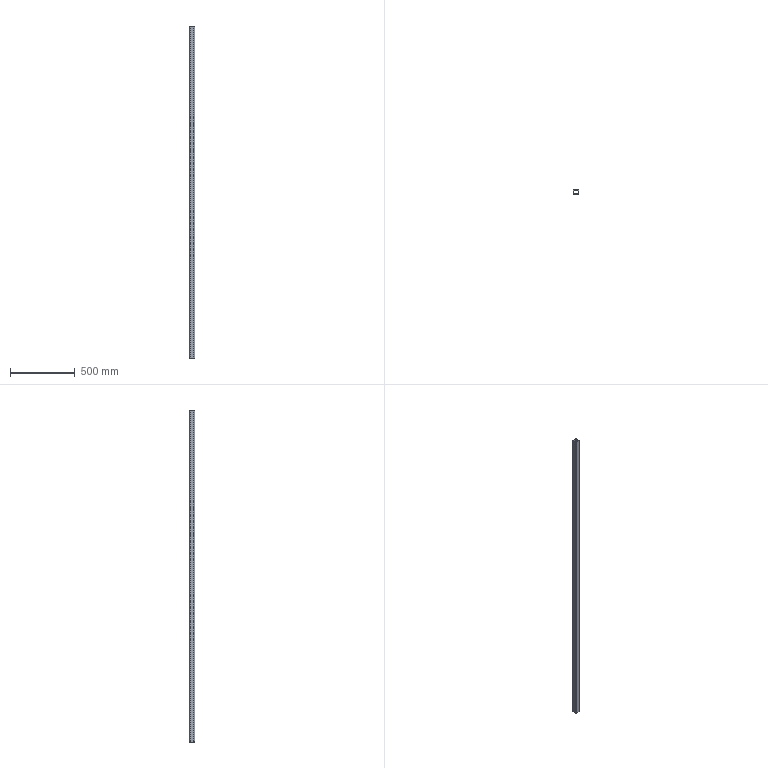Part | STEP file | body floor longitudinal beam--000.001--20240926 | 1 solid | 18 faces | box 40 x 40 x 2554 mm | volume 1074782 mm3 | plane 10 | cylinder 8 | commonest cylinder face diameters 6 x4 12 x4
STEP:
#1=CARTESIAN_POINT('',(0.,0.,0.));
#2=DIRECTION('',(0.,0.,1.));
#3=DIRECTION('',(1.,0.,0.));
#4=AXIS2_PLACEMENT_3D('',#1,#2,#3);
#5=CARTESIAN_POINT('',(-40.,149.,-50.));
#6=VERTEX_POINT('',#5);
#7=CARTESIAN_POINT('',(-40.,121.,-50.));
#8=VERTEX_POINT('',#7);
#9=CARTESIAN_POINT('',(-40.,155.,-50.));
#10=DIRECTION('',(0.,-1.,0.));
#11=VECTOR('',#10,1.);
#12=LINE('',#9,#11);
#13=CARTESIAN_POINT('',(-87.,-42.,-50.));
#14=DIRECTION('',(0.,0.,1.));
#15=DIRECTION('',(0.,-1.,0.));
#16=AXIS2_PLACEMENT_3D('',#13,#14,#15);
#17=PLANE('',#16);
#18=CARTESIAN_POINT('',(-197.,47.));
#19=DIRECTION('',(1.,0.));
#20=VECTOR('',#19,1.);
#21=LINE('',#18,#20);
#22=(GEOMETRIC_REPRESENTATION_CONTEXT(2)PARAMETRIC_REPRESENTATION_CONTEXT()REPRESENTATION_CONTEXT('',''));
#23=DEFINITIONAL_REPRESENTATION('',(#21),#22);
#24=PCURVE('',#17,#23);
#25=CARTESIAN_POINT('',(-40.,155.,2262.838));
#26=DIRECTION('',(1.,0.,0.));
#27=DIRECTION('',(0.,0.,1.));
#28=AXIS2_PLACEMENT_3D('',#25,#26,#27);
#29=PLANE('',#28);
#30=CARTESIAN_POINT('',(-2312.838,0.));
#31=DIRECTION('',(0.,1.));
#32=VECTOR('',#31,1.);
#33=LINE('',#30,#32);
#34=(GEOMETRIC_REPRESENTATION_CONTEXT(2)PARAMETRIC_REPRESENTATION_CONTEXT()REPRESENTATION_CONTEXT('',''));
#35=DEFINITIONAL_REPRESENTATION('',(#33),#34);
#36=PCURVE('',#29,#35);
#37=SURFACE_CURVE('',#12,(#24,#36),.PCURVE_S1.);
#38=EDGE_CURVE('',#6,#8,#37,.T.);
#39=ORIENTED_EDGE('',*,*,#38,.T.);
#40=CARTESIAN_POINT('',(-37.,118.,-50.));
#41=VERTEX_POINT('',#40);
#42=CARTESIAN_POINT('',(-37.,121.,-50.));
#43=DIRECTION('',(0.,0.,1.));
#44=DIRECTION('',(1.,0.,0.));
#45=AXIS2_PLACEMENT_3D('',#42,#43,#44);
#46=CIRCLE('',#45,3.);
#47=CARTESIAN_POINT('',(-163.,50.));
#48=DIRECTION('',(0.,1.));
#49=AXIS2_PLACEMENT_2D('',#47,#48);
#50=CIRCLE('',#49,3.);
#51=(GEOMETRIC_REPRESENTATION_CONTEXT(2)PARAMETRIC_REPRESENTATION_CONTEXT()REPRESENTATION_CONTEXT('',''));
#52=DEFINITIONAL_REPRESENTATION('',(#50),#51);
#53=PCURVE('',#17,#52);
#54=CARTESIAN_POINT('',(-37.,121.,2262.838));
#55=DIRECTION('',(0.,0.,1.));
#56=DIRECTION('',(-1.,0.,0.));
#57=AXIS2_PLACEMENT_3D('',#54,#55,#56);
#58=CYLINDRICAL_SURFACE('',#57,3.);
#59=CARTESIAN_POINT('',(-3.142,-2312.838));
#60=DIRECTION('',(1.,0.));
#61=VECTOR('',#60,1.);
#62=LINE('',#59,#61);
#63=(GEOMETRIC_REPRESENTATION_CONTEXT(2)PARAMETRIC_REPRESENTATION_CONTEXT()REPRESENTATION_CONTEXT('',''));
#64=DEFINITIONAL_REPRESENTATION('',(#62),#63);
#65=PCURVE('',#58,#64);
#66=SURFACE_CURVE('',#46,(#53,#65),.PCURVE_S1.);
#67=EDGE_CURVE('',#8,#41,#66,.T.);
#68=ORIENTED_EDGE('',*,*,#67,.T.);
#69=CARTESIAN_POINT('',(-9.,118.,-50.));
#70=VERTEX_POINT('',#69);
#71=CARTESIAN_POINT('',(-43.,118.,-50.));
#72=DIRECTION('',(1.,0.,0.));
#73=VECTOR('',#72,1.);
#74=LINE('',#71,#73);
#75=CARTESIAN_POINT('',(-160.,44.));
#76=DIRECTION('',(0.,1.));
#77=VECTOR('',#76,1.);
#78=LINE('',#75,#77);
#79=(GEOMETRIC_REPRESENTATION_CONTEXT(2)PARAMETRIC_REPRESENTATION_CONTEXT()REPRESENTATION_CONTEXT('',''));
#80=DEFINITIONAL_REPRESENTATION('',(#78),#79);
#81=PCURVE('',#17,#80);
#82=CARTESIAN_POINT('',(-43.,118.,2262.838));
#83=DIRECTION('',(0.,1.,0.));
#84=DIRECTION('',(0.2756,0.,-0.9613));
#85=AXIS2_PLACEMENT_3D('',#82,#83,#84);
#86=PLANE('',#85);
#87=CARTESIAN_POINT('',(2223.243,637.505));
#88=DIRECTION('',(0.2756,-0.9613));
#89=VECTOR('',#88,1.);
#90=LINE('',#87,#89);
#91=(GEOMETRIC_REPRESENTATION_CONTEXT(2)PARAMETRIC_REPRESENTATION_CONTEXT()REPRESENTATION_CONTEXT('',''));
#92=DEFINITIONAL_REPRESENTATION('',(#90),#91);
#93=PCURVE('',#86,#92);
#94=SURFACE_CURVE('',#74,(#81,#93),.PCURVE_S1.);
#95=EDGE_CURVE('',#41,#70,#94,.T.);
#96=ORIENTED_EDGE('',*,*,#95,.T.);
#97=CARTESIAN_POINT('',(-6.,121.,-50.));
#98=VERTEX_POINT('',#97);
#99=CARTESIAN_POINT('',(-9.,121.,-50.));
#100=DIRECTION('',(0.,0.,1.));
#101=DIRECTION('',(1.,0.,0.));
#102=AXIS2_PLACEMENT_3D('',#99,#100,#101);
#103=CIRCLE('',#102,3.);
#104=CARTESIAN_POINT('',(-163.,78.));
#105=DIRECTION('',(0.,1.));
#106=AXIS2_PLACEMENT_2D('',#104,#105);
#107=CIRCLE('',#106,3.);
#108=(GEOMETRIC_REPRESENTATION_CONTEXT(2)PARAMETRIC_REPRESENTATION_CONTEXT()REPRESENTATION_CONTEXT('',''));
#109=DEFINITIONAL_REPRESENTATION('',(#107),#108);
#110=PCURVE('',#17,#109);
#111=CARTESIAN_POINT('',(-9.,121.,2262.838));
#112=DIRECTION('',(0.,0.,1.));
#113=DIRECTION('',(-1.,0.,0.));
#114=AXIS2_PLACEMENT_3D('',#111,#112,#113);
#115=CYLINDRICAL_SURFACE('',#114,3.);
#116=CARTESIAN_POINT('',(-3.142,-2312.838));
#117=DIRECTION('',(1.,0.));
#118=VECTOR('',#117,1.);
#119=LINE('',#116,#118);
#120=(GEOMETRIC_REPRESENTATION_CONTEXT(2)PARAMETRIC_REPRESENTATION_CONTEXT()REPRESENTATION_CONTEXT('',''));
#121=DEFINITIONAL_REPRESENTATION('',(#119),#120);
#122=PCURVE('',#115,#121);
#123=SURFACE_CURVE('',#103,(#110,#122),.PCURVE_S1.);
#124=EDGE_CURVE('',#70,#98,#123,.T.);
#125=ORIENTED_EDGE('',*,*,#124,.T.);
#126=CARTESIAN_POINT('',(-6.,149.,-50.));
#127=VERTEX_POINT('',#126);
#128=CARTESIAN_POINT('',(-6.,115.,-50.));
#129=DIRECTION('',(0.,1.,0.));
#130=VECTOR('',#129,1.);
#131=LINE('',#128,#130);
#132=CARTESIAN_POINT('',(-157.,81.));
#133=DIRECTION('',(-1.,0.));
#134=VECTOR('',#133,1.);
#135=LINE('',#132,#134);
#136=(GEOMETRIC_REPRESENTATION_CONTEXT(2)PARAMETRIC_REPRESENTATION_CONTEXT()REPRESENTATION_CONTEXT('',''));
#137=DEFINITIONAL_REPRESENTATION('',(#135),#136);
#138=PCURVE('',#17,#137);
#139=CARTESIAN_POINT('',(-6.,115.,2262.838));
#140=DIRECTION('',(-1.,0.,0.));
#141=DIRECTION('',(0.,0.,-1.));
#142=AXIS2_PLACEMENT_3D('',#139,#140,#141);
#143=PLANE('',#142);
#144=CARTESIAN_POINT('',(2312.838,0.));
#145=DIRECTION('',(0.,-1.));
#146=VECTOR('',#145,1.);
#147=LINE('',#144,#146);
#148=(GEOMETRIC_REPRESENTATION_CONTEXT(2)PARAMETRIC_REPRESENTATION_CONTEXT()REPRESENTATION_CONTEXT('',''));
#149=DEFINITIONAL_REPRESENTATION('',(#147),#148);
#150=PCURVE('',#143,#149);
#151=SURFACE_CURVE('',#131,(#138,#150),.PCURVE_S1.);
#152=EDGE_CURVE('',#98,#127,#151,.T.);
#153=ORIENTED_EDGE('',*,*,#152,.T.);
#154=CARTESIAN_POINT('',(-9.,152.,-50.));
#155=VERTEX_POINT('',#154);
#156=CARTESIAN_POINT('',(-9.,149.,-50.));
#157=DIRECTION('',(0.,0.,1.));
#158=DIRECTION('',(1.,0.,0.));
#159=AXIS2_PLACEMENT_3D('',#156,#157,#158);
#160=CIRCLE('',#159,3.);
#161=CARTESIAN_POINT('',(-191.,78.));
#162=DIRECTION('',(0.,1.));
#163=AXIS2_PLACEMENT_2D('',#161,#162);
#164=CIRCLE('',#163,3.);
#165=(GEOMETRIC_REPRESENTATION_CONTEXT(2)PARAMETRIC_REPRESENTATION_CONTEXT()REPRESENTATION_CONTEXT('',''));
#166=DEFINITIONAL_REPRESENTATION('',(#164),#165);
#167=PCURVE('',#17,#166);
#168=CARTESIAN_POINT('',(-9.,149.,2262.838));
#169=DIRECTION('',(0.,0.,1.));
#170=DIRECTION('',(-1.,0.,0.));
#171=AXIS2_PLACEMENT_3D('',#168,#169,#170);
#172=CYLINDRICAL_SURFACE('',#171,3.);
#173=CARTESIAN_POINT('',(3.142,-2312.838));
#174=DIRECTION('',(1.,0.));
#175=VECTOR('',#174,1.);
#176=LINE('',#173,#175);
#177=(GEOMETRIC_REPRESENTATION_CONTEXT(2)PARAMETRIC_REPRESENTATION_CONTEXT()REPRESENTATION_CONTEXT('',''));
#178=DEFINITIONAL_REPRESENTATION('',(#176),#177);
#179=PCURVE('',#172,#178);
#180=SURFACE_CURVE('',#160,(#167,#179),.PCURVE_S1.);
#181=EDGE_CURVE('',#127,#155,#180,.T.);
#182=ORIENTED_EDGE('',*,*,#181,.T.);
#183=CARTESIAN_POINT('',(-37.,152.,-50.));
#184=VERTEX_POINT('',#183);
#185=CARTESIAN_POINT('',(-3.,152.,-50.));
#186=DIRECTION('',(-1.,0.,0.));
#187=VECTOR('',#186,1.);
#188=LINE('',#185,#187);
#189=CARTESIAN_POINT('',(-194.,84.));
#190=DIRECTION('',(0.,-1.));
#191=VECTOR('',#190,1.);
#192=LINE('',#189,#191);
#193=(GEOMETRIC_REPRESENTATION_CONTEXT(2)PARAMETRIC_REPRESENTATION_CONTEXT()REPRESENTATION_CONTEXT('',''));
#194=DEFINITIONAL_REPRESENTATION('',(#192),#193);
#195=PCURVE('',#17,#194);
#196=CARTESIAN_POINT('',(-3.,152.,2262.838));
#197=DIRECTION('',(0.,-1.,0.));
#198=DIRECTION('',(-0.2756,0.,0.9613));
#199=AXIS2_PLACEMENT_3D('',#196,#197,#198);
#200=PLANE('',#199);
#201=CARTESIAN_POINT('',(-2223.243,637.505));
#202=DIRECTION('',(0.2756,0.9613));
#203=VECTOR('',#202,1.);
#204=LINE('',#201,#203);
#205=(GEOMETRIC_REPRESENTATION_CONTEXT(2)PARAMETRIC_REPRESENTATION_CONTEXT()REPRESENTATION_CONTEXT('',''));
#206=DEFINITIONAL_REPRESENTATION('',(#204),#205);
#207=PCURVE('',#200,#206);
#208=SURFACE_CURVE('',#188,(#195,#207),.PCURVE_S1.);
#209=EDGE_CURVE('',#155,#184,#208,.T.);
#210=ORIENTED_EDGE('',*,*,#209,.T.);
#211=CARTESIAN_POINT('',(-37.,149.,-50.));
#212=DIRECTION('',(0.,0.,1.));
#213=DIRECTION('',(1.,0.,0.));
#214=AXIS2_PLACEMENT_3D('',#211,#212,#213);
#215=CIRCLE('',#214,3.);
#216=CARTESIAN_POINT('',(-191.,50.));
#217=DIRECTION('',(0.,1.));
#218=AXIS2_PLACEMENT_2D('',#216,#217);
#219=CIRCLE('',#218,3.);
#220=(GEOMETRIC_REPRESENTATION_CONTEXT(2)PARAMETRIC_REPRESENTATION_CONTEXT()REPRESENTATION_CONTEXT('',''));
#221=DEFINITIONAL_REPRESENTATION('',(#219),#220);
#222=PCURVE('',#17,#221);
#223=CARTESIAN_POINT('',(-37.,149.,2262.838));
#224=DIRECTION('',(0.,0.,1.));
#225=DIRECTION('',(-1.,0.,0.));
#226=AXIS2_PLACEMENT_3D('',#223,#224,#225);
#227=CYLINDRICAL_SURFACE('',#226,3.);
#228=CARTESIAN_POINT('',(3.142,-2312.838));
#229=DIRECTION('',(1.,0.));
#230=VECTOR('',#229,1.);
#231=LINE('',#228,#230);
#232=(GEOMETRIC_REPRESENTATION_CONTEXT(2)PARAMETRIC_REPRESENTATION_CONTEXT()REPRESENTATION_CONTEXT('',''));
#233=DEFINITIONAL_REPRESENTATION('',(#231),#232);
#234=PCURVE('',#227,#233);
#235=SURFACE_CURVE('',#215,(#222,#234),.PCURVE_S1.);
#236=EDGE_CURVE('',#184,#6,#235,.T.);
#237=ORIENTED_EDGE('',*,*,#236,.T.);
#238=EDGE_LOOP('',(#39,#68,#96,#125,#153,#182,#210,#237));
#239=FACE_BOUND('',#238,.T.);
#240=CARTESIAN_POINT('',(-3.,121.,-50.));
#241=VERTEX_POINT('',#240);
#242=CARTESIAN_POINT('',(-3.,149.,-50.));
#243=VERTEX_POINT('',#242);
#244=CARTESIAN_POINT('',(-3.,115.,-50.));
#245=DIRECTION('',(0.,1.,0.));
#246=VECTOR('',#245,1.);
#247=LINE('',#244,#246);
#248=CARTESIAN_POINT('',(-157.,84.));
#249=DIRECTION('',(-1.,0.));
#250=VECTOR('',#249,1.);
#251=LINE('',#248,#250);
#252=(GEOMETRIC_REPRESENTATION_CONTEXT(2)PARAMETRIC_REPRESENTATION_CONTEXT()REPRESENTATION_CONTEXT('',''));
#253=DEFINITIONAL_REPRESENTATION('',(#251),#252);
#254=PCURVE('',#17,#253);
#255=CARTESIAN_POINT('',(-3.,115.,2262.838));
#256=DIRECTION('',(-1.,0.,0.));
#257=DIRECTION('',(0.,0.,-1.));
#258=AXIS2_PLACEMENT_3D('',#255,#256,#257);
#259=PLANE('',#258);
#260=CARTESIAN_POINT('',(2312.838,0.));
#261=DIRECTION('',(0.,-1.));
#262=VECTOR('',#261,1.);
#263=LINE('',#260,#262);
#264=(GEOMETRIC_REPRESENTATION_CONTEXT(2)PARAMETRIC_REPRESENTATION_CONTEXT()REPRESENTATION_CONTEXT('',''));
#265=DEFINITIONAL_REPRESENTATION('',(#263),#264);
#266=PCURVE('',#259,#265);
#267=SURFACE_CURVE('',#247,(#254,#266),.PCURVE_S1.);
#268=EDGE_CURVE('',#241,#243,#267,.T.);
#269=ORIENTED_EDGE('',*,*,#268,.F.);
#270=CARTESIAN_POINT('',(-9.,115.,-50.));
#271=VERTEX_POINT('',#270);
#272=CARTESIAN_POINT('',(-9.,121.,-50.));
#273=DIRECTION('',(0.,0.,-1.));
#274=DIRECTION('',(1.,0.,0.));
#275=AXIS2_PLACEMENT_3D('',#272,#273,#274);
#276=CIRCLE('',#275,6.);
#277=CARTESIAN_POINT('',(-163.,84.));
#278=CARTESIAN_POINT('',(-152.608,84.));
#279=CARTESIAN_POINT('',(-157.804,75.));
#280=CARTESIAN_POINT('',(-163.,66.));
#281=CARTESIAN_POINT('',(-168.196,75.));
#282=CARTESIAN_POINT('',(-173.392,84.));
#283=CARTESIAN_POINT('',(-163.,84.));
#284=(BOUNDED_CURVE()B_SPLINE_CURVE(2,(#277,#278,#279,#280,#281,#282,#283),.UNSPECIFIED.,.T.,.F.)B_SPLINE_CURVE_WITH_KNOTS((1,2,2,2,2,1),(-2.094,0.,2.094,4.189,6.283,8.378),.UNSPECIFIED.)CURVE()GEOMETRIC_REPRESENTATION_ITEM()RATIONAL_B_SPLINE_CURVE((1.,0.5,1.,0.5,1.,0.5,1.))REPRESENTATION_ITEM(''));
#285=(GEOMETRIC_REPRESENTATION_CONTEXT(2)PARAMETRIC_REPRESENTATION_CONTEXT()REPRESENTATION_CONTEXT('',''));
#286=DEFINITIONAL_REPRESENTATION('',(#284),#285);
#287=PCURVE('',#17,#286);
#288=CARTESIAN_POINT('',(-9.,121.,2262.838));
#289=DIRECTION('',(0.,0.,1.));
#290=DIRECTION('',(-1.,0.,0.));
#291=AXIS2_PLACEMENT_3D('',#288,#289,#290);
#292=CYLINDRICAL_SURFACE('',#291,6.);
#293=CARTESIAN_POINT('',(3.142,-2312.838));
#294=DIRECTION('',(-1.,0.));
#295=VECTOR('',#294,1.);
#296=LINE('',#293,#295);
#297=(GEOMETRIC_REPRESENTATION_CONTEXT(2)PARAMETRIC_REPRESENTATION_CONTEXT()REPRESENTATION_CONTEXT('',''));
#298=DEFINITIONAL_REPRESENTATION('',(#296),#297);
#299=PCURVE('',#292,#298);
#300=SURFACE_CURVE('',#276,(#287,#299),.PCURVE_S1.);
#301=EDGE_CURVE('',#241,#271,#300,.T.);
#302=ORIENTED_EDGE('',*,*,#301,.T.);
#303=CARTESIAN_POINT('',(-37.,115.,-50.));
#304=VERTEX_POINT('',#303);
#305=CARTESIAN_POINT('',(-43.,115.,-50.));
#306=DIRECTION('',(1.,0.,0.));
#307=VECTOR('',#306,1.);
#308=LINE('',#305,#307);
#309=CARTESIAN_POINT('',(-157.,44.));
#310=DIRECTION('',(0.,1.));
#311=VECTOR('',#310,1.);
#312=LINE('',#309,#311);
#313=(GEOMETRIC_REPRESENTATION_CONTEXT(2)PARAMETRIC_REPRESENTATION_CONTEXT()REPRESENTATION_CONTEXT('',''));
#314=DEFINITIONAL_REPRESENTATION('',(#312),#313);
#315=PCURVE('',#17,#314);
#316=CARTESIAN_POINT('',(-43.,115.,2262.838));
#317=DIRECTION('',(0.,1.,0.));
#318=DIRECTION('',(0.2756,0.,-0.9613));
#319=AXIS2_PLACEMENT_3D('',#316,#317,#318);
#320=PLANE('',#319);
#321=CARTESIAN_POINT('',(2223.243,637.505));
#322=DIRECTION('',(0.2756,-0.9613));
#323=VECTOR('',#322,1.);
#324=LINE('',#321,#323);
#325=(GEOMETRIC_REPRESENTATION_CONTEXT(2)PARAMETRIC_REPRESENTATION_CONTEXT()REPRESENTATION_CONTEXT('',''));
#326=DEFINITIONAL_REPRESENTATION('',(#324),#325);
#327=PCURVE('',#320,#326);
#328=SURFACE_CURVE('',#308,(#315,#327),.PCURVE_S1.);
#329=EDGE_CURVE('',#304,#271,#328,.T.);
#330=ORIENTED_EDGE('',*,*,#329,.F.);
#331=CARTESIAN_POINT('',(-43.,121.,-50.));
#332=VERTEX_POINT('',#331);
#333=CARTESIAN_POINT('',(-37.,121.,-50.));
#334=DIRECTION('',(0.,0.,-1.));
#335=DIRECTION('',(1.,0.,0.));
#336=AXIS2_PLACEMENT_3D('',#333,#334,#335);
#337=CIRCLE('',#336,6.);
#338=CARTESIAN_POINT('',(-163.,56.));
#339=CARTESIAN_POINT('',(-152.608,56.));
#340=CARTESIAN_POINT('',(-157.804,47.));
#341=CARTESIAN_POINT('',(-163.,38.));
#342=CARTESIAN_POINT('',(-168.196,47.));
#343=CARTESIAN_POINT('',(-173.392,56.));
#344=CARTESIAN_POINT('',(-163.,56.));
#345=(BOUNDED_CURVE()B_SPLINE_CURVE(2,(#338,#339,#340,#341,#342,#343,#344),.UNSPECIFIED.,.T.,.F.)B_SPLINE_CURVE_WITH_KNOTS((1,2,2,2,2,1),(-2.094,0.,2.094,4.189,6.283,8.378),.UNSPECIFIED.)CURVE()GEOMETRIC_REPRESENTATION_ITEM()RATIONAL_B_SPLINE_CURVE((1.,0.5,1.,0.5,1.,0.5,1.))REPRESENTATION_ITEM(''));
#346=(GEOMETRIC_REPRESENTATION_CONTEXT(2)PARAMETRIC_REPRESENTATION_CONTEXT()REPRESENTATION_CONTEXT('',''));
#347=DEFINITIONAL_REPRESENTATION('',(#345),#346);
#348=PCURVE('',#17,#347);
#349=CARTESIAN_POINT('',(-37.,121.,2262.838));
#350=DIRECTION('',(0.,0.,1.));
#351=DIRECTION('',(-1.,0.,0.));
#352=AXIS2_PLACEMENT_3D('',#349,#350,#351);
#353=CYLINDRICAL_SURFACE('',#352,6.);
#354=CARTESIAN_POINT('',(3.142,-2312.838));
#355=DIRECTION('',(-1.,0.));
#356=VECTOR('',#355,1.);
#357=LINE('',#354,#356);
#358=(GEOMETRIC_REPRESENTATION_CONTEXT(2)PARAMETRIC_REPRESENTATION_CONTEXT()REPRESENTATION_CONTEXT('',''));
#359=DEFINITIONAL_REPRESENTATION('',(#357),#358);
#360=PCURVE('',#353,#359);
#361=SURFACE_CURVE('',#337,(#348,#360),.PCURVE_S1.);
#362=EDGE_CURVE('',#304,#332,#361,.T.);
#363=ORIENTED_EDGE('',*,*,#362,.T.);
#364=CARTESIAN_POINT('',(-43.,149.,-50.));
#365=VERTEX_POINT('',#364);
#366=CARTESIAN_POINT('',(-43.,155.,-50.));
#367=DIRECTION('',(0.,-1.,0.));
#368=VECTOR('',#367,1.);
#369=LINE('',#366,#368);
#370=CARTESIAN_POINT('',(-197.,44.));
#371=DIRECTION('',(1.,0.));
#372=VECTOR('',#371,1.);
#373=LINE('',#370,#372);
#374=(GEOMETRIC_REPRESENTATION_CONTEXT(2)PARAMETRIC_REPRESENTATION_CONTEXT()REPRESENTATION_CONTEXT('',''));
#375=DEFINITIONAL_REPRESENTATION('',(#373),#374);
#376=PCURVE('',#17,#375);
#377=CARTESIAN_POINT('',(-43.,155.,2262.838));
#378=DIRECTION('',(1.,0.,0.));
#379=DIRECTION('',(0.,0.,1.));
#380=AXIS2_PLACEMENT_3D('',#377,#378,#379);
#381=PLANE('',#380);
#382=CARTESIAN_POINT('',(-2312.838,0.));
#383=DIRECTION('',(0.,1.));
#384=VECTOR('',#383,1.);
#385=LINE('',#382,#384);
#386=(GEOMETRIC_REPRESENTATION_CONTEXT(2)PARAMETRIC_REPRESENTATION_CONTEXT()REPRESENTATION_CONTEXT('',''));
#387=DEFINITIONAL_REPRESENTATION('',(#385),#386);
#388=PCURVE('',#381,#387);
#389=SURFACE_CURVE('',#369,(#376,#388),.PCURVE_S1.);
#390=EDGE_CURVE('',#365,#332,#389,.T.);
#391=ORIENTED_EDGE('',*,*,#390,.F.);
#392=CARTESIAN_POINT('',(-37.,155.,-50.));
#393=VERTEX_POINT('',#392);
#394=CARTESIAN_POINT('',(-37.,149.,-50.));
#395=DIRECTION('',(0.,0.,-1.));
#396=DIRECTION('',(1.,0.,0.));
#397=AXIS2_PLACEMENT_3D('',#394,#395,#396);
#398=CIRCLE('',#397,6.);
#399=CARTESIAN_POINT('',(-191.,56.));
#400=CARTESIAN_POINT('',(-180.608,56.));
#401=CARTESIAN_POINT('',(-185.804,47.));
#402=CARTESIAN_POINT('',(-191.,38.));
#403=CARTESIAN_POINT('',(-196.196,47.));
#404=CARTESIAN_POINT('',(-201.392,56.));
#405=CARTESIAN_POINT('',(-191.,56.));
#406=(BOUNDED_CURVE()B_SPLINE_CURVE(2,(#399,#400,#401,#402,#403,#404,#405),.UNSPECIFIED.,.T.,.F.)B_SPLINE_CURVE_WITH_KNOTS((1,2,2,2,2,1),(-2.094,0.,2.094,4.189,6.283,8.378),.UNSPECIFIED.)CURVE()GEOMETRIC_REPRESENTATION_ITEM()RATIONAL_B_SPLINE_CURVE((1.,0.5,1.,0.5,1.,0.5,1.))REPRESENTATION_ITEM(''));
#407=(GEOMETRIC_REPRESENTATION_CONTEXT(2)PARAMETRIC_REPRESENTATION_CONTEXT()REPRESENTATION_CONTEXT('',''));
#408=DEFINITIONAL_REPRESENTATION('',(#406),#407);
#409=PCURVE('',#17,#408);
#410=CARTESIAN_POINT('',(-37.,149.,2262.838));
#411=DIRECTION('',(0.,0.,1.));
#412=DIRECTION('',(-1.,0.,0.));
#413=AXIS2_PLACEMENT_3D('',#410,#411,#412);
#414=CYLINDRICAL_SURFACE('',#413,6.);
#415=CARTESIAN_POINT('',(9.425,-2312.838));
#416=DIRECTION('',(-1.,0.));
#417=VECTOR('',#416,1.);
#418=LINE('',#415,#417);
#419=(GEOMETRIC_REPRESENTATION_CONTEXT(2)PARAMETRIC_REPRESENTATION_CONTEXT()REPRESENTATION_CONTEXT('',''));
#420=DEFINITIONAL_REPRESENTATION('',(#418),#419);
#421=PCURVE('',#414,#420);
#422=SURFACE_CURVE('',#398,(#409,#421),.PCURVE_S1.);
#423=EDGE_CURVE('',#365,#393,#422,.T.);
#424=ORIENTED_EDGE('',*,*,#423,.T.);
#425=CARTESIAN_POINT('',(-9.,155.,-50.));
#426=VERTEX_POINT('',#425);
#427=CARTESIAN_POINT('',(-3.,155.,-50.));
#428=DIRECTION('',(-1.,0.,0.));
#429=VECTOR('',#428,1.);
#430=LINE('',#427,#429);
#431=CARTESIAN_POINT('',(-197.,84.));
#432=DIRECTION('',(0.,-1.));
#433=VECTOR('',#432,1.);
#434=LINE('',#431,#433);
#435=(GEOMETRIC_REPRESENTATION_CONTEXT(2)PARAMETRIC_REPRESENTATION_CONTEXT()REPRESENTATION_CONTEXT('',''));
#436=DEFINITIONAL_REPRESENTATION('',(#434),#435);
#437=PCURVE('',#17,#436);
#438=CARTESIAN_POINT('',(-3.,155.,2262.838));
#439=DIRECTION('',(0.,-1.,0.));
#440=DIRECTION('',(-0.2756,0.,0.9613));
#441=AXIS2_PLACEMENT_3D('',#438,#439,#440);
#442=PLANE('',#441);
#443=CARTESIAN_POINT('',(-2223.243,637.505));
#444=DIRECTION('',(0.2756,0.9613));
#445=VECTOR('',#444,1.);
#446=LINE('',#443,#445);
#447=(GEOMETRIC_REPRESENTATION_CONTEXT(2)PARAMETRIC_REPRESENTATION_CONTEXT()REPRESENTATION_CONTEXT('',''));
#448=DEFINITIONAL_REPRESENTATION('',(#446),#447);
#449=PCURVE('',#442,#448);
#450=SURFACE_CURVE('',#430,(#437,#449),.PCURVE_S1.);
#451=EDGE_CURVE('',#426,#393,#450,.T.);
#452=ORIENTED_EDGE('',*,*,#451,.F.);
#453=CARTESIAN_POINT('',(-9.,149.,-50.));
#454=DIRECTION('',(0.,0.,-1.));
#455=DIRECTION('',(1.,0.,0.));
#456=AXIS2_PLACEMENT_3D('',#453,#454,#455);
#457=CIRCLE('',#456,6.);
#458=CARTESIAN_POINT('',(-191.,84.));
#459=CARTESIAN_POINT('',(-180.608,84.));
#460=CARTESIAN_POINT('',(-185.804,75.));
#461=CARTESIAN_POINT('',(-191.,66.));
#462=CARTESIAN_POINT('',(-196.196,75.));
#463=CARTESIAN_POINT('',(-201.392,84.));
#464=CARTESIAN_POINT('',(-191.,84.));
#465=(BOUNDED_CURVE()B_SPLINE_CURVE(2,(#458,#459,#460,#461,#462,#463,#464),.UNSPECIFIED.,.T.,.F.)B_SPLINE_CURVE_WITH_KNOTS((1,2,2,2,2,1),(-2.094,0.,2.094,4.189,6.283,8.378),.UNSPECIFIED.)CURVE()GEOMETRIC_REPRESENTATION_ITEM()RATIONAL_B_SPLINE_CURVE((1.,0.5,1.,0.5,1.,0.5,1.))REPRESENTATION_ITEM(''));
#466=(GEOMETRIC_REPRESENTATION_CONTEXT(2)PARAMETRIC_REPRESENTATION_CONTEXT()REPRESENTATION_CONTEXT('',''));
#467=DEFINITIONAL_REPRESENTATION('',(#465),#466);
#468=PCURVE('',#17,#467);
#469=CARTESIAN_POINT('',(-9.,149.,2262.838));
#470=DIRECTION('',(0.,0.,1.));
#471=DIRECTION('',(-1.,0.,0.));
#472=AXIS2_PLACEMENT_3D('',#469,#470,#471);
#473=CYLINDRICAL_SURFACE('',#472,6.);
#474=CARTESIAN_POINT('',(9.425,-2312.838));
#475=DIRECTION('',(-1.,0.));
#476=VECTOR('',#475,1.);
#477=LINE('',#474,#476);
#478=(GEOMETRIC_REPRESENTATION_CONTEXT(2)PARAMETRIC_REPRESENTATION_CONTEXT()REPRESENTATION_CONTEXT('',''));
#479=DEFINITIONAL_REPRESENTATION('',(#477),#478);
#480=PCURVE('',#473,#479);
#481=SURFACE_CURVE('',#457,(#468,#480),.PCURVE_S1.);
#482=EDGE_CURVE('',#426,#243,#481,.T.);
#483=ORIENTED_EDGE('',*,*,#482,.T.);
#484=EDGE_LOOP('',(#269,#302,#330,#363,#391,#424,#452,#483));
#485=FACE_BOUND('',#484,.T.);
#486=ADVANCED_FACE('',(#239,#485),#17,.F.);
#487=CARTESIAN_POINT('',(-37.,118.,2504.));
#488=VERTEX_POINT('',#487);
#489=CARTESIAN_POINT('',(-9.,118.,2504.));
#490=VERTEX_POINT('',#489);
#491=CARTESIAN_POINT('',(-43.,118.,2504.));
#492=DIRECTION('',(1.,0.,0.));
#493=VECTOR('',#492,1.);
#494=LINE('',#491,#493);
#495=CARTESIAN_POINT('',(-112.,92.,2504.));
#496=DIRECTION('',(0.,0.,1.));
#497=DIRECTION('',(0.,1.,0.));
#498=AXIS2_PLACEMENT_3D('',#495,#496,#497);
#499=PLANE('',#498);
#500=CARTESIAN_POINT('',(26.,-69.));
#501=DIRECTION('',(0.,-1.));
#502=VECTOR('',#501,1.);
#503=LINE('',#500,#502);
#504=(GEOMETRIC_REPRESENTATION_CONTEXT(2)PARAMETRIC_REPRESENTATION_CONTEXT()REPRESENTATION_CONTEXT('',''));
#505=DEFINITIONAL_REPRESENTATION('',(#503),#504);
#506=PCURVE('',#499,#505);
#507=CARTESIAN_POINT('',(-231.819,-66.473));
#508=DIRECTION('',(0.2756,-0.9613));
#509=VECTOR('',#508,1.);
#510=LINE('',#507,#509);
#511=(GEOMETRIC_REPRESENTATION_CONTEXT(2)PARAMETRIC_REPRESENTATION_CONTEXT()REPRESENTATION_CONTEXT('',''));
#512=DEFINITIONAL_REPRESENTATION('',(#510),#511);
#513=PCURVE('',#86,#512);
#514=SURFACE_CURVE('',#494,(#506,#513),.PCURVE_S1.);
#515=EDGE_CURVE('',#488,#490,#514,.T.);
#516=ORIENTED_EDGE('',*,*,#515,.F.);
#517=CARTESIAN_POINT('',(-40.,121.,2504.));
#518=VERTEX_POINT('',#517);
#519=CARTESIAN_POINT('',(-37.,121.,2504.));
#520=DIRECTION('',(0.,0.,-1.));
#521=DIRECTION('',(1.,0.,0.));
#522=AXIS2_PLACEMENT_3D('',#519,#520,#521);
#523=CIRCLE('',#522,3.);
#524=CARTESIAN_POINT('',(29.,-78.));
#525=CARTESIAN_POINT('',(23.804,-78.));
#526=CARTESIAN_POINT('',(26.402,-73.5));
#527=CARTESIAN_POINT('',(29.,-69.));
#528=CARTESIAN_POINT('',(31.598,-73.5));
#529=CARTESIAN_POINT('',(34.196,-78.));
#530=CARTESIAN_POINT('',(29.,-78.));
#531=(BOUNDED_CURVE()B_SPLINE_CURVE(2,(#524,#525,#526,#527,#528,#529,#530),.UNSPECIFIED.,.T.,.F.)B_SPLINE_CURVE_WITH_KNOTS((1,2,2,2,2,1),(-2.094,0.,2.094,4.189,6.283,8.378),.UNSPECIFIED.)CURVE()GEOMETRIC_REPRESENTATION_ITEM()RATIONAL_B_SPLINE_CURVE((1.,0.5,1.,0.5,1.,0.5,1.))REPRESENTATION_ITEM(''));
#532=(GEOMETRIC_REPRESENTATION_CONTEXT(2)PARAMETRIC_REPRESENTATION_CONTEXT()REPRESENTATION_CONTEXT('',''));
#533=DEFINITIONAL_REPRESENTATION('',(#531),#532);
#534=PCURVE('',#499,#533);
#535=CARTESIAN_POINT('',(3.142,241.162));
#536=DIRECTION('',(-1.,0.));
#537=VECTOR('',#536,1.);
#538=LINE('',#535,#537);
#539=(GEOMETRIC_REPRESENTATION_CONTEXT(2)PARAMETRIC_REPRESENTATION_CONTEXT()REPRESENTATION_CONTEXT('',''));
#540=DEFINITIONAL_REPRESENTATION('',(#538),#539);
#541=PCURVE('',#58,#540);
#542=SURFACE_CURVE('',#523,(#534,#541),.PCURVE_S1.);
#543=EDGE_CURVE('',#488,#518,#542,.T.);
#544=ORIENTED_EDGE('',*,*,#543,.T.);
#545=CARTESIAN_POINT('',(-40.,149.,2504.));
#546=VERTEX_POINT('',#545);
#547=CARTESIAN_POINT('',(-40.,155.,2504.));
#548=DIRECTION('',(0.,-1.,0.));
#549=VECTOR('',#548,1.);
#550=LINE('',#547,#549);
#551=CARTESIAN_POINT('',(63.,-72.));
#552=DIRECTION('',(-1.,0.));
#553=VECTOR('',#552,1.);
#554=LINE('',#551,#553);
#555=(GEOMETRIC_REPRESENTATION_CONTEXT(2)PARAMETRIC_REPRESENTATION_CONTEXT()REPRESENTATION_CONTEXT('',''));
#556=DEFINITIONAL_REPRESENTATION('',(#554),#555);
#557=PCURVE('',#499,#556);
#558=CARTESIAN_POINT('',(241.162,0.));
#559=DIRECTION('',(0.,1.));
#560=VECTOR('',#559,1.);
#561=LINE('',#558,#560);
#562=(GEOMETRIC_REPRESENTATION_CONTEXT(2)PARAMETRIC_REPRESENTATION_CONTEXT()REPRESENTATION_CONTEXT('',''));
#563=DEFINITIONAL_REPRESENTATION('',(#561),#562);
#564=PCURVE('',#29,#563);
#565=SURFACE_CURVE('',#550,(#557,#564),.PCURVE_S1.);
#566=EDGE_CURVE('',#546,#518,#565,.T.);
#567=ORIENTED_EDGE('',*,*,#566,.F.);
#568=CARTESIAN_POINT('',(-37.,152.,2504.));
#569=VERTEX_POINT('',#568);
#570=CARTESIAN_POINT('',(-37.,149.,2504.));
#571=DIRECTION('',(0.,0.,-1.));
#572=DIRECTION('',(1.,0.,0.));
#573=AXIS2_PLACEMENT_3D('',#570,#571,#572);
#574=CIRCLE('',#573,3.);
#575=CARTESIAN_POINT('',(57.,-78.));
#576=CARTESIAN_POINT('',(51.804,-78.));
#577=CARTESIAN_POINT('',(54.402,-73.5));
#578=CARTESIAN_POINT('',(57.,-69.));
#579=CARTESIAN_POINT('',(59.598,-73.5));
#580=CARTESIAN_POINT('',(62.196,-78.));
#581=CARTESIAN_POINT('',(57.,-78.));
#582=(BOUNDED_CURVE()B_SPLINE_CURVE(2,(#575,#576,#577,#578,#579,#580,#581),.UNSPECIFIED.,.T.,.F.)B_SPLINE_CURVE_WITH_KNOTS((1,2,2,2,2,1),(-2.094,0.,2.094,4.189,6.283,8.378),.UNSPECIFIED.)CURVE()GEOMETRIC_REPRESENTATION_ITEM()RATIONAL_B_SPLINE_CURVE((1.,0.5,1.,0.5,1.,0.5,1.))REPRESENTATION_ITEM(''));
#583=(GEOMETRIC_REPRESENTATION_CONTEXT(2)PARAMETRIC_REPRESENTATION_CONTEXT()REPRESENTATION_CONTEXT('',''));
#584=DEFINITIONAL_REPRESENTATION('',(#582),#583);
#585=PCURVE('',#499,#584);
#586=CARTESIAN_POINT('',(9.425,241.162));
#587=DIRECTION('',(-1.,0.));
#588=VECTOR('',#587,1.);
#589=LINE('',#586,#588);
#590=(GEOMETRIC_REPRESENTATION_CONTEXT(2)PARAMETRIC_REPRESENTATION_CONTEXT()REPRESENTATION_CONTEXT('',''));
#591=DEFINITIONAL_REPRESENTATION('',(#589),#590);
#592=PCURVE('',#227,#591);
#593=SURFACE_CURVE('',#574,(#585,#592),.PCURVE_S1.);
#594=EDGE_CURVE('',#546,#569,#593,.T.);
#595=ORIENTED_EDGE('',*,*,#594,.T.);
#596=CARTESIAN_POINT('',(-9.,152.,2504.));
#597=VERTEX_POINT('',#596);
#598=CARTESIAN_POINT('',(-3.,152.,2504.));
#599=DIRECTION('',(-1.,0.,0.));
#600=VECTOR('',#599,1.);
#601=LINE('',#598,#600);
#602=CARTESIAN_POINT('',(60.,-109.));
#603=DIRECTION('',(0.,1.));
#604=VECTOR('',#603,1.);
#605=LINE('',#602,#604);
#606=(GEOMETRIC_REPRESENTATION_CONTEXT(2)PARAMETRIC_REPRESENTATION_CONTEXT()REPRESENTATION_CONTEXT('',''));
#607=DEFINITIONAL_REPRESENTATION('',(#605),#606);
#608=PCURVE('',#499,#607);
#609=CARTESIAN_POINT('',(231.819,-66.473));
#610=DIRECTION('',(0.2756,0.9613));
#611=VECTOR('',#610,1.);
#612=LINE('',#609,#611);
#613=(GEOMETRIC_REPRESENTATION_CONTEXT(2)PARAMETRIC_REPRESENTATION_CONTEXT()REPRESENTATION_CONTEXT('',''));
#614=DEFINITIONAL_REPRESENTATION('',(#612),#613);
#615=PCURVE('',#200,#614);
#616=SURFACE_CURVE('',#601,(#608,#615),.PCURVE_S1.);
#617=EDGE_CURVE('',#597,#569,#616,.T.);
#618=ORIENTED_EDGE('',*,*,#617,.F.);
#619=CARTESIAN_POINT('',(-6.,149.,2504.));
#620=VERTEX_POINT('',#619);
#621=CARTESIAN_POINT('',(-9.,149.,2504.));
#622=DIRECTION('',(0.,0.,-1.));
#623=DIRECTION('',(1.,0.,0.));
#624=AXIS2_PLACEMENT_3D('',#621,#622,#623);
#625=CIRCLE('',#624,3.);
#626=CARTESIAN_POINT('',(57.,-106.));
#627=CARTESIAN_POINT('',(51.804,-106.));
#628=CARTESIAN_POINT('',(54.402,-101.5));
#629=CARTESIAN_POINT('',(57.,-97.));
#630=CARTESIAN_POINT('',(59.598,-101.5));
#631=CARTESIAN_POINT('',(62.196,-106.));
#632=CARTESIAN_POINT('',(57.,-106.));
#633=(BOUNDED_CURVE()B_SPLINE_CURVE(2,(#626,#627,#628,#629,#630,#631,#632),.UNSPECIFIED.,.T.,.F.)B_SPLINE_CURVE_WITH_KNOTS((1,2,2,2,2,1),(-2.094,0.,2.094,4.189,6.283,8.378),.UNSPECIFIED.)CURVE()GEOMETRIC_REPRESENTATION_ITEM()RATIONAL_B_SPLINE_CURVE((1.,0.5,1.,0.5,1.,0.5,1.))REPRESENTATION_ITEM(''));
#634=(GEOMETRIC_REPRESENTATION_CONTEXT(2)PARAMETRIC_REPRESENTATION_CONTEXT()REPRESENTATION_CONTEXT('',''));
#635=DEFINITIONAL_REPRESENTATION('',(#633),#634);
#636=PCURVE('',#499,#635);
#637=CARTESIAN_POINT('',(9.425,241.162));
#638=DIRECTION('',(-1.,0.));
#639=VECTOR('',#638,1.);
#640=LINE('',#637,#639);
#641=(GEOMETRIC_REPRESENTATION_CONTEXT(2)PARAMETRIC_REPRESENTATION_CONTEXT()REPRESENTATION_CONTEXT('',''));
#642=DEFINITIONAL_REPRESENTATION('',(#640),#641);
#643=PCURVE('',#172,#642);
#644=SURFACE_CURVE('',#625,(#636,#643),.PCURVE_S1.);
#645=EDGE_CURVE('',#597,#620,#644,.T.);
#646=ORIENTED_EDGE('',*,*,#645,.T.);
#647=CARTESIAN_POINT('',(-6.,121.,2504.));
#648=VERTEX_POINT('',#647);
#649=CARTESIAN_POINT('',(-6.,115.,2504.));
#650=DIRECTION('',(0.,1.,0.));
#651=VECTOR('',#650,1.);
#652=LINE('',#649,#651);
#653=CARTESIAN_POINT('',(23.,-106.));
#654=DIRECTION('',(1.,0.));
#655=VECTOR('',#654,1.);
#656=LINE('',#653,#655);
#657=(GEOMETRIC_REPRESENTATION_CONTEXT(2)PARAMETRIC_REPRESENTATION_CONTEXT()REPRESENTATION_CONTEXT('',''));
#658=DEFINITIONAL_REPRESENTATION('',(#656),#657);
#659=PCURVE('',#499,#658);
#660=CARTESIAN_POINT('',(-241.162,0.));
#661=DIRECTION('',(0.,-1.));
#662=VECTOR('',#661,1.);
#663=LINE('',#660,#662);
#664=(GEOMETRIC_REPRESENTATION_CONTEXT(2)PARAMETRIC_REPRESENTATION_CONTEXT()REPRESENTATION_CONTEXT('',''));
#665=DEFINITIONAL_REPRESENTATION('',(#663),#664);
#666=PCURVE('',#143,#665);
#667=SURFACE_CURVE('',#652,(#659,#666),.PCURVE_S1.);
#668=EDGE_CURVE('',#648,#620,#667,.T.);
#669=ORIENTED_EDGE('',*,*,#668,.F.);
#670=CARTESIAN_POINT('',(-9.,121.,2504.));
#671=DIRECTION('',(0.,0.,-1.));
#672=DIRECTION('',(1.,0.,0.));
#673=AXIS2_PLACEMENT_3D('',#670,#671,#672);
#674=CIRCLE('',#673,3.);
#675=CARTESIAN_POINT('',(29.,-106.));
#676=CARTESIAN_POINT('',(23.804,-106.));
#677=CARTESIAN_POINT('',(26.402,-101.5));
#678=CARTESIAN_POINT('',(29.,-97.));
#679=CARTESIAN_POINT('',(31.598,-101.5));
#680=CARTESIAN_POINT('',(34.196,-106.));
#681=CARTESIAN_POINT('',(29.,-106.));
#682=(BOUNDED_CURVE()B_SPLINE_CURVE(2,(#675,#676,#677,#678,#679,#680,#681),.UNSPECIFIED.,.T.,.F.)B_SPLINE_CURVE_WITH_KNOTS((1,2,2,2,2,1),(-2.094,0.,2.094,4.189,6.283,8.378),.UNSPECIFIED.)CURVE()GEOMETRIC_REPRESENTATION_ITEM()RATIONAL_B_SPLINE_CURVE((1.,0.5,1.,0.5,1.,0.5,1.))REPRESENTATION_ITEM(''));
#683=(GEOMETRIC_REPRESENTATION_CONTEXT(2)PARAMETRIC_REPRESENTATION_CONTEXT()REPRESENTATION_CONTEXT('',''));
#684=DEFINITIONAL_REPRESENTATION('',(#682),#683);
#685=PCURVE('',#499,#684);
#686=CARTESIAN_POINT('',(3.142,241.162));
#687=DIRECTION('',(-1.,0.));
#688=VECTOR('',#687,1.);
#689=LINE('',#686,#688);
#690=(GEOMETRIC_REPRESENTATION_CONTEXT(2)PARAMETRIC_REPRESENTATION_CONTEXT()REPRESENTATION_CONTEXT('',''));
#691=DEFINITIONAL_REPRESENTATION('',(#689),#690);
#692=PCURVE('',#115,#691);
#693=SURFACE_CURVE('',#674,(#685,#692),.PCURVE_S1.);
#694=EDGE_CURVE('',#648,#490,#693,.T.);
#695=ORIENTED_EDGE('',*,*,#694,.T.);
#696=EDGE_LOOP('',(#516,#544,#567,#595,#618,#646,#669,#695));
#697=FACE_BOUND('',#696,.T.);
#698=CARTESIAN_POINT('',(-37.,115.,2504.));
#699=VERTEX_POINT('',#698);
#700=CARTESIAN_POINT('',(-9.,115.,2504.));
#701=VERTEX_POINT('',#700);
#702=CARTESIAN_POINT('',(-43.,115.,2504.));
#703=DIRECTION('',(1.,0.,0.));
#704=VECTOR('',#703,1.);
#705=LINE('',#702,#704);
#706=CARTESIAN_POINT('',(23.,-69.));
#707=DIRECTION('',(0.,-1.));
#708=VECTOR('',#707,1.);
#709=LINE('',#706,#708);
#710=(GEOMETRIC_REPRESENTATION_CONTEXT(2)PARAMETRIC_REPRESENTATION_CONTEXT()REPRESENTATION_CONTEXT('',''));
#711=DEFINITIONAL_REPRESENTATION('',(#709),#710);
#712=PCURVE('',#499,#711);
#713=CARTESIAN_POINT('',(-231.819,-66.473));
#714=DIRECTION('',(0.2756,-0.9613));
#715=VECTOR('',#714,1.);
#716=LINE('',#713,#715);
#717=(GEOMETRIC_REPRESENTATION_CONTEXT(2)PARAMETRIC_REPRESENTATION_CONTEXT()REPRESENTATION_CONTEXT('',''));
#718=DEFINITIONAL_REPRESENTATION('',(#716),#717);
#719=PCURVE('',#320,#718);
#720=SURFACE_CURVE('',#705,(#712,#719),.PCURVE_S1.);
#721=EDGE_CURVE('',#699,#701,#720,.T.);
#722=ORIENTED_EDGE('',*,*,#721,.T.);
#723=CARTESIAN_POINT('',(-3.,121.,2504.));
#724=VERTEX_POINT('',#723);
#725=CARTESIAN_POINT('',(-9.,121.,2504.));
#726=DIRECTION('',(0.,0.,1.));
#727=DIRECTION('',(1.,0.,0.));
#728=AXIS2_PLACEMENT_3D('',#725,#726,#727);
#729=CIRCLE('',#728,6.);
#730=CARTESIAN_POINT('',(29.,-103.));
#731=DIRECTION('',(0.,-1.));
#732=AXIS2_PLACEMENT_2D('',#730,#731);
#733=CIRCLE('',#732,6.);
#734=(GEOMETRIC_REPRESENTATION_CONTEXT(2)PARAMETRIC_REPRESENTATION_CONTEXT()REPRESENTATION_CONTEXT('',''));
#735=DEFINITIONAL_REPRESENTATION('',(#733),#734);
#736=PCURVE('',#499,#735);
#737=CARTESIAN_POINT('',(-3.142,241.162));
#738=DIRECTION('',(1.,0.));
#739=VECTOR('',#738,1.);
#740=LINE('',#737,#739);
#741=(GEOMETRIC_REPRESENTATION_CONTEXT(2)PARAMETRIC_REPRESENTATION_CONTEXT()REPRESENTATION_CONTEXT('',''));
#742=DEFINITIONAL_REPRESENTATION('',(#740),#741);
#743=PCURVE('',#292,#742);
#744=SURFACE_CURVE('',#729,(#736,#743),.PCURVE_S1.);
#745=EDGE_CURVE('',#701,#724,#744,.T.);
#746=ORIENTED_EDGE('',*,*,#745,.T.);
#747=CARTESIAN_POINT('',(-3.,149.,2504.));
#748=VERTEX_POINT('',#747);
#749=CARTESIAN_POINT('',(-3.,115.,2504.));
#750=DIRECTION('',(0.,1.,0.));
#751=VECTOR('',#750,1.);
#752=LINE('',#749,#751);
#753=CARTESIAN_POINT('',(23.,-109.));
#754=DIRECTION('',(1.,0.));
#755=VECTOR('',#754,1.);
#756=LINE('',#753,#755);
#757=(GEOMETRIC_REPRESENTATION_CONTEXT(2)PARAMETRIC_REPRESENTATION_CONTEXT()REPRESENTATION_CONTEXT('',''));
#758=DEFINITIONAL_REPRESENTATION('',(#756),#757);
#759=PCURVE('',#499,#758);
#760=CARTESIAN_POINT('',(-241.162,0.));
#761=DIRECTION('',(0.,-1.));
#762=VECTOR('',#761,1.);
#763=LINE('',#760,#762);
#764=(GEOMETRIC_REPRESENTATION_CONTEXT(2)PARAMETRIC_REPRESENTATION_CONTEXT()REPRESENTATION_CONTEXT('',''));
#765=DEFINITIONAL_REPRESENTATION('',(#763),#764);
#766=PCURVE('',#259,#765);
#767=SURFACE_CURVE('',#752,(#759,#766),.PCURVE_S1.);
#768=EDGE_CURVE('',#724,#748,#767,.T.);
#769=ORIENTED_EDGE('',*,*,#768,.T.);
#770=CARTESIAN_POINT('',(-9.,155.,2504.));
#771=VERTEX_POINT('',#770);
#772=CARTESIAN_POINT('',(-9.,149.,2504.));
#773=DIRECTION('',(0.,0.,1.));
#774=DIRECTION('',(1.,0.,0.));
#775=AXIS2_PLACEMENT_3D('',#772,#773,#774);
#776=CIRCLE('',#775,6.);
#777=CARTESIAN_POINT('',(57.,-103.));
#778=DIRECTION('',(0.,-1.));
#779=AXIS2_PLACEMENT_2D('',#777,#778);
#780=CIRCLE('',#779,6.);
#781=(GEOMETRIC_REPRESENTATION_CONTEXT(2)PARAMETRIC_REPRESENTATION_CONTEXT()REPRESENTATION_CONTEXT('',''));
#782=DEFINITIONAL_REPRESENTATION('',(#780),#781);
#783=PCURVE('',#499,#782);
#784=CARTESIAN_POINT('',(3.142,241.162));
#785=DIRECTION('',(1.,0.));
#786=VECTOR('',#785,1.);
#787=LINE('',#784,#786);
#788=(GEOMETRIC_REPRESENTATION_CONTEXT(2)PARAMETRIC_REPRESENTATION_CONTEXT()REPRESENTATION_CONTEXT('',''));
#789=DEFINITIONAL_REPRESENTATION('',(#787),#788);
#790=PCURVE('',#473,#789);
#791=SURFACE_CURVE('',#776,(#783,#790),.PCURVE_S1.);
#792=EDGE_CURVE('',#748,#771,#791,.T.);
#793=ORIENTED_EDGE('',*,*,#792,.T.);
#794=CARTESIAN_POINT('',(-37.,155.,2504.));
#795=VERTEX_POINT('',#794);
#796=CARTESIAN_POINT('',(-3.,155.,2504.));
#797=DIRECTION('',(-1.,0.,0.));
#798=VECTOR('',#797,1.);
#799=LINE('',#796,#798);
#800=CARTESIAN_POINT('',(63.,-109.));
#801=DIRECTION('',(0.,1.));
#802=VECTOR('',#801,1.);
#803=LINE('',#800,#802);
#804=(GEOMETRIC_REPRESENTATION_CONTEXT(2)PARAMETRIC_REPRESENTATION_CONTEXT()REPRESENTATION_CONTEXT('',''));
#805=DEFINITIONAL_REPRESENTATION('',(#803),#804);
#806=PCURVE('',#499,#805);
#807=CARTESIAN_POINT('',(231.819,-66.473));
#808=DIRECTION('',(0.2756,0.9613));
#809=VECTOR('',#808,1.);
#810=LINE('',#807,#809);
#811=(GEOMETRIC_REPRESENTATION_CONTEXT(2)PARAMETRIC_REPRESENTATION_CONTEXT()REPRESENTATION_CONTEXT('',''));
#812=DEFINITIONAL_REPRESENTATION('',(#810),#811);
#813=PCURVE('',#442,#812);
#814=SURFACE_CURVE('',#799,(#806,#813),.PCURVE_S1.);
#815=EDGE_CURVE('',#771,#795,#814,.T.);
#816=ORIENTED_EDGE('',*,*,#815,.T.);
#817=CARTESIAN_POINT('',(-43.,149.,2504.));
#818=VERTEX_POINT('',#817);
#819=CARTESIAN_POINT('',(-37.,149.,2504.));
#820=DIRECTION('',(0.,0.,1.));
#821=DIRECTION('',(1.,0.,0.));
#822=AXIS2_PLACEMENT_3D('',#819,#820,#821);
#823=CIRCLE('',#822,6.);
#824=CARTESIAN_POINT('',(57.,-75.));
#825=DIRECTION('',(0.,-1.));
#826=AXIS2_PLACEMENT_2D('',#824,#825);
#827=CIRCLE('',#826,6.);
#828=(GEOMETRIC_REPRESENTATION_CONTEXT(2)PARAMETRIC_REPRESENTATION_CONTEXT()REPRESENTATION_CONTEXT('',''));
#829=DEFINITIONAL_REPRESENTATION('',(#827),#828);
#830=PCURVE('',#499,#829);
#831=CARTESIAN_POINT('',(3.142,241.162));
#832=DIRECTION('',(1.,0.));
#833=VECTOR('',#832,1.);
#834=LINE('',#831,#833);
#835=(GEOMETRIC_REPRESENTATION_CONTEXT(2)PARAMETRIC_REPRESENTATION_CONTEXT()REPRESENTATION_CONTEXT('',''));
#836=DEFINITIONAL_REPRESENTATION('',(#834),#835);
#837=PCURVE('',#414,#836);
#838=SURFACE_CURVE('',#823,(#830,#837),.PCURVE_S1.);
#839=EDGE_CURVE('',#795,#818,#838,.T.);
#840=ORIENTED_EDGE('',*,*,#839,.T.);
#841=CARTESIAN_POINT('',(-43.,121.,2504.));
#842=VERTEX_POINT('',#841);
#843=CARTESIAN_POINT('',(-43.,155.,2504.));
#844=DIRECTION('',(0.,-1.,0.));
#845=VECTOR('',#844,1.);
#846=LINE('',#843,#845);
#847=CARTESIAN_POINT('',(63.,-69.));
#848=DIRECTION('',(-1.,0.));
#849=VECTOR('',#848,1.);
#850=LINE('',#847,#849);
#851=(GEOMETRIC_REPRESENTATION_CONTEXT(2)PARAMETRIC_REPRESENTATION_CONTEXT()REPRESENTATION_CONTEXT('',''));
#852=DEFINITIONAL_REPRESENTATION('',(#850),#851);
#853=PCURVE('',#499,#852);
#854=CARTESIAN_POINT('',(241.162,0.));
#855=DIRECTION('',(0.,1.));
#856=VECTOR('',#855,1.);
#857=LINE('',#854,#856);
#858=(GEOMETRIC_REPRESENTATION_CONTEXT(2)PARAMETRIC_REPRESENTATION_CONTEXT()REPRESENTATION_CONTEXT('',''));
#859=DEFINITIONAL_REPRESENTATION('',(#857),#858);
#860=PCURVE('',#381,#859);
#861=SURFACE_CURVE('',#846,(#853,#860),.PCURVE_S1.);
#862=EDGE_CURVE('',#818,#842,#861,.T.);
#863=ORIENTED_EDGE('',*,*,#862,.T.);
#864=CARTESIAN_POINT('',(-37.,121.,2504.));
#865=DIRECTION('',(0.,0.,1.));
#866=DIRECTION('',(1.,0.,0.));
#867=AXIS2_PLACEMENT_3D('',#864,#865,#866);
#868=CIRCLE('',#867,6.);
#869=CARTESIAN_POINT('',(29.,-75.));
#870=DIRECTION('',(0.,-1.));
#871=AXIS2_PLACEMENT_2D('',#869,#870);
#872=CIRCLE('',#871,6.);
#873=(GEOMETRIC_REPRESENTATION_CONTEXT(2)PARAMETRIC_REPRESENTATION_CONTEXT()REPRESENTATION_CONTEXT('',''));
#874=DEFINITIONAL_REPRESENTATION('',(#872),#873);
#875=PCURVE('',#499,#874);
#876=CARTESIAN_POINT('',(-3.142,241.162));
#877=DIRECTION('',(1.,0.));
#878=VECTOR('',#877,1.);
#879=LINE('',#876,#878);
#880=(GEOMETRIC_REPRESENTATION_CONTEXT(2)PARAMETRIC_REPRESENTATION_CONTEXT()REPRESENTATION_CONTEXT('',''));
#881=DEFINITIONAL_REPRESENTATION('',(#879),#880);
#882=PCURVE('',#353,#881);
#883=SURFACE_CURVE('',#868,(#875,#882),.PCURVE_S1.);
#884=EDGE_CURVE('',#842,#699,#883,.T.);
#885=ORIENTED_EDGE('',*,*,#884,.T.);
#886=EDGE_LOOP('',(#722,#746,#769,#793,#816,#840,#863,#885));
#887=FACE_BOUND('',#886,.T.);
#888=ADVANCED_FACE('',(#697,#887),#499,.T.);
#889=ORIENTED_EDGE('',*,*,#95,.F.);
#890=CARTESIAN_POINT('',(-37.,118.,2504.));
#891=DIRECTION('',(0.,0.,1.));
#892=VECTOR('',#891,1.);
#893=LINE('',#890,#892);
#894=CARTESIAN_POINT('',(-230.166,-72.241));
#895=DIRECTION('',(-0.9613,-0.2756));
#896=VECTOR('',#895,1.);
#897=LINE('',#894,#896);
#898=(GEOMETRIC_REPRESENTATION_CONTEXT(2)PARAMETRIC_REPRESENTATION_CONTEXT()REPRESENTATION_CONTEXT('',''));
#899=DEFINITIONAL_REPRESENTATION('',(#897),#898);
#900=PCURVE('',#86,#899);
#901=CARTESIAN_POINT('',(1.571,241.162));
#902=DIRECTION('',(0.,1.));
#903=VECTOR('',#902,1.);
#904=LINE('',#901,#903);
#905=(GEOMETRIC_REPRESENTATION_CONTEXT(2)PARAMETRIC_REPRESENTATION_CONTEXT()REPRESENTATION_CONTEXT('',''));
#906=DEFINITIONAL_REPRESENTATION('',(#904),#905);
#907=PCURVE('',#58,#906);
#908=SURFACE_CURVE('',#893,(#900,#907),.PCURVE_S1.);
#909=EDGE_CURVE('',#41,#488,#908,.T.);
#910=ORIENTED_EDGE('',*,*,#909,.T.);
#911=ORIENTED_EDGE('',*,*,#515,.T.);
#912=CARTESIAN_POINT('',(-9.,118.,0.));
#913=DIRECTION('',(0.,0.,-1.));
#914=VECTOR('',#913,1.);
#915=LINE('',#912,#914);
#916=CARTESIAN_POINT('',(2184.552,591.04));
#917=DIRECTION('',(0.9613,0.2756));
#918=VECTOR('',#917,1.);
#919=LINE('',#916,#918);
#920=(GEOMETRIC_REPRESENTATION_CONTEXT(2)PARAMETRIC_REPRESENTATION_CONTEXT()REPRESENTATION_CONTEXT('',''));
#921=DEFINITIONAL_REPRESENTATION('',(#919),#920);
#922=PCURVE('',#86,#921);
#923=CARTESIAN_POINT('',(1.571,-2262.838));
#924=DIRECTION('',(0.,-1.));
#925=VECTOR('',#924,1.);
#926=LINE('',#923,#925);
#927=(GEOMETRIC_REPRESENTATION_CONTEXT(2)PARAMETRIC_REPRESENTATION_CONTEXT()REPRESENTATION_CONTEXT('',''));
#928=DEFINITIONAL_REPRESENTATION('',(#926),#927);
#929=PCURVE('',#115,#928);
#930=SURFACE_CURVE('',#915,(#922,#929),.PCURVE_S1.);
#931=EDGE_CURVE('',#490,#70,#930,.T.);
#932=ORIENTED_EDGE('',*,*,#931,.T.);
#933=EDGE_LOOP('',(#889,#910,#911,#932));
#934=FACE_BOUND('',#933,.T.);
#935=ADVANCED_FACE('',(#934),#86,.T.);
#936=ORIENTED_EDGE('',*,*,#152,.F.);
#937=CARTESIAN_POINT('',(-6.,121.,2504.));
#938=DIRECTION('',(0.,0.,1.));
#939=VECTOR('',#938,1.);
#940=LINE('',#937,#939);
#941=CARTESIAN_POINT('',(-241.162,-6.));
#942=DIRECTION('',(-1.,0.));
#943=VECTOR('',#942,1.);
#944=LINE('',#941,#943);
#945=(GEOMETRIC_REPRESENTATION_CONTEXT(2)PARAMETRIC_REPRESENTATION_CONTEXT()REPRESENTATION_CONTEXT('',''));
#946=DEFINITIONAL_REPRESENTATION('',(#944),#945);
#947=PCURVE('',#143,#946);
#948=CARTESIAN_POINT('',(3.142,241.162));
#949=DIRECTION('',(0.,1.));
#950=VECTOR('',#949,1.);
#951=LINE('',#948,#950);
#952=(GEOMETRIC_REPRESENTATION_CONTEXT(2)PARAMETRIC_REPRESENTATION_CONTEXT()REPRESENTATION_CONTEXT('',''));
#953=DEFINITIONAL_REPRESENTATION('',(#951),#952);
#954=PCURVE('',#115,#953);
#955=SURFACE_CURVE('',#940,(#947,#954),.PCURVE_S1.);
#956=EDGE_CURVE('',#98,#648,#955,.T.);
#957=ORIENTED_EDGE('',*,*,#956,.T.);
#958=ORIENTED_EDGE('',*,*,#668,.T.);
#959=CARTESIAN_POINT('',(-6.,149.,0.));
#960=DIRECTION('',(0.,0.,-1.));
#961=VECTOR('',#960,1.);
#962=LINE('',#959,#961);
#963=CARTESIAN_POINT('',(2262.838,-34.));
#964=DIRECTION('',(1.,0.));
#965=VECTOR('',#964,1.);
#966=LINE('',#963,#965);
#967=(GEOMETRIC_REPRESENTATION_CONTEXT(2)PARAMETRIC_REPRESENTATION_CONTEXT()REPRESENTATION_CONTEXT('',''));
#968=DEFINITIONAL_REPRESENTATION('',(#966),#967);
#969=PCURVE('',#143,#968);
#970=CARTESIAN_POINT('',(3.142,-2262.838));
#971=DIRECTION('',(0.,-1.));
#972=VECTOR('',#971,1.);
#973=LINE('',#970,#972);
#974=(GEOMETRIC_REPRESENTATION_CONTEXT(2)PARAMETRIC_REPRESENTATION_CONTEXT()REPRESENTATION_CONTEXT('',''));
#975=DEFINITIONAL_REPRESENTATION('',(#973),#974);
#976=PCURVE('',#172,#975);
#977=SURFACE_CURVE('',#962,(#969,#976),.PCURVE_S1.);
#978=EDGE_CURVE('',#620,#127,#977,.T.);
#979=ORIENTED_EDGE('',*,*,#978,.T.);
#980=EDGE_LOOP('',(#936,#957,#958,#979));
#981=FACE_BOUND('',#980,.T.);
#982=ADVANCED_FACE('',(#981),#143,.T.);
#983=ORIENTED_EDGE('',*,*,#209,.F.);
#984=CARTESIAN_POINT('',(-9.,152.,2504.));
#985=DIRECTION('',(0.,0.,1.));
#986=VECTOR('',#985,1.);
#987=LINE('',#984,#986);
#988=CARTESIAN_POINT('',(233.473,-60.706));
#989=DIRECTION('',(0.9613,-0.2756));
#990=VECTOR('',#989,1.);
#991=LINE('',#988,#990);
#992=(GEOMETRIC_REPRESENTATION_CONTEXT(2)PARAMETRIC_REPRESENTATION_CONTEXT()REPRESENTATION_CONTEXT('',''));
#993=DEFINITIONAL_REPRESENTATION('',(#991),#992);
#994=PCURVE('',#200,#993);
#995=CARTESIAN_POINT('',(4.712,241.162));
#996=DIRECTION('',(0.,1.));
#997=VECTOR('',#996,1.);
#998=LINE('',#995,#997);
#999=(GEOMETRIC_REPRESENTATION_CONTEXT(2)PARAMETRIC_REPRESENTATION_CONTEXT()REPRESENTATION_CONTEXT('',''));
#1000=DEFINITIONAL_REPRESENTATION('',(#998),#999);
#1001=PCURVE('',#172,#1000);
#1002=SURFACE_CURVE('',#987,(#994,#1001),.PCURVE_S1.);
#1003=EDGE_CURVE('',#155,#597,#1002,.T.);
#1004=ORIENTED_EDGE('',*,*,#1003,.T.);
#1005=ORIENTED_EDGE('',*,*,#617,.T.);
#1006=CARTESIAN_POINT('',(-37.,152.,0.));
#1007=DIRECTION('',(0.,0.,-1.));
#1008=VECTOR('',#1007,1.);
#1009=LINE('',#1006,#1008);
#1010=CARTESIAN_POINT('',(-2165.808,656.406));
#1011=DIRECTION('',(-0.9613,0.2756));
#1012=VECTOR('',#1011,1.);
#1013=LINE('',#1010,#1012);
#1014=(GEOMETRIC_REPRESENTATION_CONTEXT(2)PARAMETRIC_REPRESENTATION_CONTEXT()REPRESENTATION_CONTEXT('',''));
#1015=DEFINITIONAL_REPRESENTATION('',(#1013),#1014);
#1016=PCURVE('',#200,#1015);
#1017=CARTESIAN_POINT('',(4.712,-2262.838));
#1018=DIRECTION('',(0.,-1.));
#1019=VECTOR('',#1018,1.);
#1020=LINE('',#1017,#1019);
#1021=(GEOMETRIC_REPRESENTATION_CONTEXT(2)PARAMETRIC_REPRESENTATION_CONTEXT()REPRESENTATION_CONTEXT('',''));
#1022=DEFINITIONAL_REPRESENTATION('',(#1020),#1021);
#1023=PCURVE('',#227,#1022);
#1024=SURFACE_CURVE('',#1009,(#1016,#1023),.PCURVE_S1.);
#1025=EDGE_CURVE('',#569,#184,#1024,.T.);
#1026=ORIENTED_EDGE('',*,*,#1025,.T.);
#1027=EDGE_LOOP('',(#983,#1004,#1005,#1026));
#1028=FACE_BOUND('',#1027,.T.);
#1029=ADVANCED_FACE('',(#1028),#200,.T.);
#1030=ORIENTED_EDGE('',*,*,#566,.T.);
#1031=CARTESIAN_POINT('',(-40.,121.,0.));
#1032=DIRECTION('',(0.,0.,-1.));
#1033=VECTOR('',#1032,1.);
#1034=LINE('',#1031,#1033);
#1035=CARTESIAN_POINT('',(-2262.838,34.));
#1036=DIRECTION('',(-1.,0.));
#1037=VECTOR('',#1036,1.);
#1038=LINE('',#1035,#1037);
#1039=(GEOMETRIC_REPRESENTATION_CONTEXT(2)PARAMETRIC_REPRESENTATION_CONTEXT()REPRESENTATION_CONTEXT('',''));
#1040=DEFINITIONAL_REPRESENTATION('',(#1038),#1039);
#1041=PCURVE('',#29,#1040);
#1042=CARTESIAN_POINT('',(0.,-2262.838));
#1043=DIRECTION('',(0.,-1.));
#1044=VECTOR('',#1043,1.);
#1045=LINE('',#1042,#1044);
#1046=(GEOMETRIC_REPRESENTATION_CONTEXT(2)PARAMETRIC_REPRESENTATION_CONTEXT()REPRESENTATION_CONTEXT('',''));
#1047=DEFINITIONAL_REPRESENTATION('',(#1045),#1046);
#1048=PCURVE('',#58,#1047);
#1049=SURFACE_CURVE('',#1034,(#1041,#1048),.PCURVE_S1.);
#1050=EDGE_CURVE('',#518,#8,#1049,.T.);
#1051=ORIENTED_EDGE('',*,*,#1050,.T.);
#1052=ORIENTED_EDGE('',*,*,#38,.F.);
#1053=CARTESIAN_POINT('',(-40.,149.,2504.));
#1054=DIRECTION('',(0.,0.,1.));
#1055=VECTOR('',#1054,1.);
#1056=LINE('',#1053,#1055);
#1057=CARTESIAN_POINT('',(241.162,6.));
#1058=DIRECTION('',(1.,0.));
#1059=VECTOR('',#1058,1.);
#1060=LINE('',#1057,#1059);
#1061=(GEOMETRIC_REPRESENTATION_CONTEXT(2)PARAMETRIC_REPRESENTATION_CONTEXT()REPRESENTATION_CONTEXT('',''));
#1062=DEFINITIONAL_REPRESENTATION('',(#1060),#1061);
#1063=PCURVE('',#29,#1062);
#1064=CARTESIAN_POINT('',(6.283,241.162));
#1065=DIRECTION('',(0.,1.));
#1066=VECTOR('',#1065,1.);
#1067=LINE('',#1064,#1066);
#1068=(GEOMETRIC_REPRESENTATION_CONTEXT(2)PARAMETRIC_REPRESENTATION_CONTEXT()REPRESENTATION_CONTEXT('',''));
#1069=DEFINITIONAL_REPRESENTATION('',(#1067),#1068);
#1070=PCURVE('',#227,#1069);
#1071=SURFACE_CURVE('',#1056,(#1063,#1070),.PCURVE_S1.);
#1072=EDGE_CURVE('',#6,#546,#1071,.T.);
#1073=ORIENTED_EDGE('',*,*,#1072,.T.);
#1074=EDGE_LOOP('',(#1030,#1051,#1052,#1073));
#1075=FACE_BOUND('',#1074,.T.);
#1076=ADVANCED_FACE('',(#1075),#29,.T.);
#1077=ORIENTED_EDGE('',*,*,#329,.T.);
#1078=CARTESIAN_POINT('',(-9.,115.,2262.838));
#1079=DIRECTION('',(0.,0.,1.));
#1080=VECTOR('',#1079,1.);
#1081=LINE('',#1078,#1080);
#1082=CARTESIAN_POINT('',(9.372,-32.683));
#1083=DIRECTION('',(-0.9613,-0.2756));
#1084=VECTOR('',#1083,1.);
#1085=LINE('',#1082,#1084);
#1086=(GEOMETRIC_REPRESENTATION_CONTEXT(2)PARAMETRIC_REPRESENTATION_CONTEXT()REPRESENTATION_CONTEXT('',''));
#1087=DEFINITIONAL_REPRESENTATION('',(#1085),#1086);
#1088=PCURVE('',#320,#1087);
#1089=CARTESIAN_POINT('',(1.571,0.));
#1090=DIRECTION('',(0.,1.));
#1091=VECTOR('',#1090,1.);
#1092=LINE('',#1089,#1091);
#1093=(GEOMETRIC_REPRESENTATION_CONTEXT(2)PARAMETRIC_REPRESENTATION_CONTEXT()REPRESENTATION_CONTEXT('',''));
#1094=DEFINITIONAL_REPRESENTATION('',(#1092),#1093);
#1095=PCURVE('',#292,#1094);
#1096=SURFACE_CURVE('',#1081,(#1088,#1095),.PCURVE_S1.);
#1097=EDGE_CURVE('',#271,#701,#1096,.T.);
#1098=ORIENTED_EDGE('',*,*,#1097,.T.);
#1099=ORIENTED_EDGE('',*,*,#721,.F.);
#1100=CARTESIAN_POINT('',(-37.,115.,2262.838));
#1101=DIRECTION('',(0.,0.,-1.));
#1102=VECTOR('',#1101,1.);
#1103=LINE('',#1100,#1102);
#1104=CARTESIAN_POINT('',(1.654,-5.768));
#1105=DIRECTION('',(0.9613,0.2756));
#1106=VECTOR('',#1105,1.);
#1107=LINE('',#1104,#1106);
#1108=(GEOMETRIC_REPRESENTATION_CONTEXT(2)PARAMETRIC_REPRESENTATION_CONTEXT()REPRESENTATION_CONTEXT('',''));
#1109=DEFINITIONAL_REPRESENTATION('',(#1107),#1108);
#1110=PCURVE('',#320,#1109);
#1111=CARTESIAN_POINT('',(1.571,0.));
#1112=DIRECTION('',(0.,-1.));
#1113=VECTOR('',#1112,1.);
#1114=LINE('',#1111,#1113);
#1115=(GEOMETRIC_REPRESENTATION_CONTEXT(2)PARAMETRIC_REPRESENTATION_CONTEXT()REPRESENTATION_CONTEXT('',''));
#1116=DEFINITIONAL_REPRESENTATION('',(#1114),#1115);
#1117=PCURVE('',#353,#1116);
#1118=SURFACE_CURVE('',#1103,(#1110,#1117),.PCURVE_S1.);
#1119=EDGE_CURVE('',#699,#304,#1118,.T.);
#1120=ORIENTED_EDGE('',*,*,#1119,.T.);
#1121=EDGE_LOOP('',(#1077,#1098,#1099,#1120));
#1122=FACE_BOUND('',#1121,.T.);
#1123=ADVANCED_FACE('',(#1122),#320,.F.);
#1124=ORIENTED_EDGE('',*,*,#768,.F.);
#1125=CARTESIAN_POINT('',(-3.,121.,2262.838));
#1126=DIRECTION('',(0.,0.,-1.));
#1127=VECTOR('',#1126,1.);
#1128=LINE('',#1125,#1127);
#1129=CARTESIAN_POINT('',(0.,-6.));
#1130=DIRECTION('',(1.,0.));
#1131=VECTOR('',#1130,1.);
#1132=LINE('',#1129,#1131);
#1133=(GEOMETRIC_REPRESENTATION_CONTEXT(2)PARAMETRIC_REPRESENTATION_CONTEXT()REPRESENTATION_CONTEXT('',''));
#1134=DEFINITIONAL_REPRESENTATION('',(#1132),#1133);
#1135=PCURVE('',#259,#1134);
#1136=CARTESIAN_POINT('',(3.142,0.));
#1137=DIRECTION('',(0.,-1.));
#1138=VECTOR('',#1137,1.);
#1139=LINE('',#1136,#1138);
#1140=(GEOMETRIC_REPRESENTATION_CONTEXT(2)PARAMETRIC_REPRESENTATION_CONTEXT()REPRESENTATION_CONTEXT('',''));
#1141=DEFINITIONAL_REPRESENTATION('',(#1139),#1140);
#1142=PCURVE('',#292,#1141);
#1143=SURFACE_CURVE('',#1128,(#1135,#1142),.PCURVE_S1.);
#1144=EDGE_CURVE('',#724,#241,#1143,.T.);
#1145=ORIENTED_EDGE('',*,*,#1144,.T.);
#1146=ORIENTED_EDGE('',*,*,#268,.T.);
#1147=CARTESIAN_POINT('',(-3.,149.,2262.838));
#1148=DIRECTION('',(0.,0.,1.));
#1149=VECTOR('',#1148,1.);
#1150=LINE('',#1147,#1149);
#1151=CARTESIAN_POINT('',(0.,-34.));
#1152=DIRECTION('',(-1.,0.));
#1153=VECTOR('',#1152,1.);
#1154=LINE('',#1151,#1153);
#1155=(GEOMETRIC_REPRESENTATION_CONTEXT(2)PARAMETRIC_REPRESENTATION_CONTEXT()REPRESENTATION_CONTEXT('',''));
#1156=DEFINITIONAL_REPRESENTATION('',(#1154),#1155);
#1157=PCURVE('',#259,#1156);
#1158=CARTESIAN_POINT('',(3.142,0.));
#1159=DIRECTION('',(0.,1.));
#1160=VECTOR('',#1159,1.);
#1161=LINE('',#1158,#1160);
#1162=(GEOMETRIC_REPRESENTATION_CONTEXT(2)PARAMETRIC_REPRESENTATION_CONTEXT()REPRESENTATION_CONTEXT('',''));
#1163=DEFINITIONAL_REPRESENTATION('',(#1161),#1162);
#1164=PCURVE('',#473,#1163);
#1165=SURFACE_CURVE('',#1150,(#1157,#1164),.PCURVE_S1.);
#1166=EDGE_CURVE('',#243,#748,#1165,.T.);
#1167=ORIENTED_EDGE('',*,*,#1166,.T.);
#1168=EDGE_LOOP('',(#1124,#1145,#1146,#1167));
#1169=FACE_BOUND('',#1168,.T.);
#1170=ADVANCED_FACE('',(#1169),#259,.F.);
#1171=ORIENTED_EDGE('',*,*,#815,.F.);
#1172=CARTESIAN_POINT('',(-9.,155.,2262.838));
#1173=DIRECTION('',(0.,0.,-1.));
#1174=VECTOR('',#1173,1.);
#1175=LINE('',#1172,#1174);
#1176=CARTESIAN_POINT('',(1.654,5.768));
#1177=DIRECTION('',(-0.9613,0.2756));
#1178=VECTOR('',#1177,1.);
#1179=LINE('',#1176,#1178);
#1180=(GEOMETRIC_REPRESENTATION_CONTEXT(2)PARAMETRIC_REPRESENTATION_CONTEXT()REPRESENTATION_CONTEXT('',''));
#1181=DEFINITIONAL_REPRESENTATION('',(#1179),#1180);
#1182=PCURVE('',#442,#1181);
#1183=CARTESIAN_POINT('',(4.712,0.));
#1184=DIRECTION('',(0.,-1.));
#1185=VECTOR('',#1184,1.);
#1186=LINE('',#1183,#1185);
#1187=(GEOMETRIC_REPRESENTATION_CONTEXT(2)PARAMETRIC_REPRESENTATION_CONTEXT()REPRESENTATION_CONTEXT('',''));
#1188=DEFINITIONAL_REPRESENTATION('',(#1186),#1187);
#1189=PCURVE('',#473,#1188);
#1190=SURFACE_CURVE('',#1175,(#1182,#1189),.PCURVE_S1.);
#1191=EDGE_CURVE('',#771,#426,#1190,.T.);
#1192=ORIENTED_EDGE('',*,*,#1191,.T.);
#1193=ORIENTED_EDGE('',*,*,#451,.T.);
#1194=CARTESIAN_POINT('',(-37.,155.,2262.838));
#1195=DIRECTION('',(0.,0.,1.));
#1196=VECTOR('',#1195,1.);
#1197=LINE('',#1194,#1196);
#1198=CARTESIAN_POINT('',(9.372,32.683));
#1199=DIRECTION('',(0.9613,-0.2756));
#1200=VECTOR('',#1199,1.);
#1201=LINE('',#1198,#1200);
#1202=(GEOMETRIC_REPRESENTATION_CONTEXT(2)PARAMETRIC_REPRESENTATION_CONTEXT()REPRESENTATION_CONTEXT('',''));
#1203=DEFINITIONAL_REPRESENTATION('',(#1201),#1202);
#1204=PCURVE('',#442,#1203);
#1205=CARTESIAN_POINT('',(4.712,0.));
#1206=DIRECTION('',(0.,1.));
#1207=VECTOR('',#1206,1.);
#1208=LINE('',#1205,#1207);
#1209=(GEOMETRIC_REPRESENTATION_CONTEXT(2)PARAMETRIC_REPRESENTATION_CONTEXT()REPRESENTATION_CONTEXT('',''));
#1210=DEFINITIONAL_REPRESENTATION('',(#1208),#1209);
#1211=PCURVE('',#414,#1210);
#1212=SURFACE_CURVE('',#1197,(#1204,#1211),.PCURVE_S1.);
#1213=EDGE_CURVE('',#393,#795,#1212,.T.);
#1214=ORIENTED_EDGE('',*,*,#1213,.T.);
#1215=EDGE_LOOP('',(#1171,#1192,#1193,#1214));
#1216=FACE_BOUND('',#1215,.T.);
#1217=ADVANCED_FACE('',(#1216),#442,.F.);
#1218=ORIENTED_EDGE('',*,*,#390,.T.);
#1219=CARTESIAN_POINT('',(-43.,121.,2262.838));
#1220=DIRECTION('',(0.,0.,1.));
#1221=VECTOR('',#1220,1.);
#1222=LINE('',#1219,#1221);
#1223=CARTESIAN_POINT('',(0.,34.));
#1224=DIRECTION('',(1.,0.));
#1225=VECTOR('',#1224,1.);
#1226=LINE('',#1223,#1225);
#1227=(GEOMETRIC_REPRESENTATION_CONTEXT(2)PARAMETRIC_REPRESENTATION_CONTEXT()REPRESENTATION_CONTEXT('',''));
#1228=DEFINITIONAL_REPRESENTATION('',(#1226),#1227);
#1229=PCURVE('',#381,#1228);
#1230=CARTESIAN_POINT('',(0.,0.));
#1231=DIRECTION('',(0.,1.));
#1232=VECTOR('',#1231,1.);
#1233=LINE('',#1230,#1232);
#1234=(GEOMETRIC_REPRESENTATION_CONTEXT(2)PARAMETRIC_REPRESENTATION_CONTEXT()REPRESENTATION_CONTEXT('',''));
#1235=DEFINITIONAL_REPRESENTATION('',(#1233),#1234);
#1236=PCURVE('',#353,#1235);
#1237=SURFACE_CURVE('',#1222,(#1229,#1236),.PCURVE_S1.);
#1238=EDGE_CURVE('',#332,#842,#1237,.T.);
#1239=ORIENTED_EDGE('',*,*,#1238,.T.);
#1240=ORIENTED_EDGE('',*,*,#862,.F.);
#1241=CARTESIAN_POINT('',(-43.,149.,2262.838));
#1242=DIRECTION('',(0.,0.,-1.));
#1243=VECTOR('',#1242,1.);
#1244=LINE('',#1241,#1243);
#1245=CARTESIAN_POINT('',(0.,6.));
#1246=DIRECTION('',(-1.,0.));
#1247=VECTOR('',#1246,1.);
#1248=LINE('',#1245,#1247);
#1249=(GEOMETRIC_REPRESENTATION_CONTEXT(2)PARAMETRIC_REPRESENTATION_CONTEXT()REPRESENTATION_CONTEXT('',''));
#1250=DEFINITIONAL_REPRESENTATION('',(#1248),#1249);
#1251=PCURVE('',#381,#1250);
#1252=CARTESIAN_POINT('',(6.283,0.));
#1253=DIRECTION('',(0.,-1.));
#1254=VECTOR('',#1253,1.);
#1255=LINE('',#1252,#1254);
#1256=(GEOMETRIC_REPRESENTATION_CONTEXT(2)PARAMETRIC_REPRESENTATION_CONTEXT()REPRESENTATION_CONTEXT('',''));
#1257=DEFINITIONAL_REPRESENTATION('',(#1255),#1256);
#1258=PCURVE('',#414,#1257);
#1259=SURFACE_CURVE('',#1244,(#1251,#1258),.PCURVE_S1.);
#1260=EDGE_CURVE('',#818,#365,#1259,.T.);
#1261=ORIENTED_EDGE('',*,*,#1260,.T.);
#1262=EDGE_LOOP('',(#1218,#1239,#1240,#1261));
#1263=FACE_BOUND('',#1262,.T.);
#1264=ADVANCED_FACE('',(#1263),#381,.F.);
#1265=ORIENTED_EDGE('',*,*,#792,.F.);
#1266=ORIENTED_EDGE('',*,*,#1166,.F.);
#1267=ORIENTED_EDGE('',*,*,#482,.F.);
#1268=ORIENTED_EDGE('',*,*,#1191,.F.);
#1269=EDGE_LOOP('',(#1265,#1266,#1267,#1268));
#1270=FACE_BOUND('',#1269,.T.);
#1271=ADVANCED_FACE('',(#1270),#473,.T.);
#1272=ORIENTED_EDGE('',*,*,#839,.F.);
#1273=ORIENTED_EDGE('',*,*,#1213,.F.);
#1274=ORIENTED_EDGE('',*,*,#423,.F.);
#1275=ORIENTED_EDGE('',*,*,#1260,.F.);
#1276=EDGE_LOOP('',(#1272,#1273,#1274,#1275));
#1277=FACE_BOUND('',#1276,.T.);
#1278=ADVANCED_FACE('',(#1277),#414,.T.);
#1279=ORIENTED_EDGE('',*,*,#884,.F.);
#1280=ORIENTED_EDGE('',*,*,#1238,.F.);
#1281=ORIENTED_EDGE('',*,*,#362,.F.);
#1282=ORIENTED_EDGE('',*,*,#1119,.F.);
#1283=EDGE_LOOP('',(#1279,#1280,#1281,#1282));
#1284=FACE_BOUND('',#1283,.T.);
#1285=ADVANCED_FACE('',(#1284),#353,.T.);
#1286=ORIENTED_EDGE('',*,*,#745,.F.);
#1287=ORIENTED_EDGE('',*,*,#1097,.F.);
#1288=ORIENTED_EDGE('',*,*,#301,.F.);
#1289=ORIENTED_EDGE('',*,*,#1144,.F.);
#1290=EDGE_LOOP('',(#1286,#1287,#1288,#1289));
#1291=FACE_BOUND('',#1290,.T.);
#1292=ADVANCED_FACE('',(#1291),#292,.T.);
#1293=ORIENTED_EDGE('',*,*,#1050,.T.);
#1294=ORIENTED_EDGE('',*,*,#67,.T.);
#1295=ORIENTED_EDGE('',*,*,#909,.T.);
#1296=ORIENTED_EDGE('',*,*,#543,.T.);
#1297=EDGE_LOOP('',(#1293,#1294,#1295,#1296));
#1298=FACE_BOUND('',#1297,.F.);
#1299=ADVANCED_FACE('',(#1298),#58,.F.);
#1300=ORIENTED_EDGE('',*,*,#931,.T.);
#1301=ORIENTED_EDGE('',*,*,#124,.T.);
#1302=ORIENTED_EDGE('',*,*,#956,.T.);
#1303=ORIENTED_EDGE('',*,*,#694,.T.);
#1304=EDGE_LOOP('',(#1300,#1301,#1302,#1303));
#1305=FACE_BOUND('',#1304,.F.);
#1306=ADVANCED_FACE('',(#1305),#115,.F.);
#1307=ORIENTED_EDGE('',*,*,#978,.T.);
#1308=ORIENTED_EDGE('',*,*,#181,.T.);
#1309=ORIENTED_EDGE('',*,*,#1003,.T.);
#1310=ORIENTED_EDGE('',*,*,#645,.T.);
#1311=EDGE_LOOP('',(#1307,#1308,#1309,#1310));
#1312=FACE_BOUND('',#1311,.F.);
#1313=ADVANCED_FACE('',(#1312),#172,.F.);
#1314=ORIENTED_EDGE('',*,*,#1025,.T.);
#1315=ORIENTED_EDGE('',*,*,#236,.T.);
#1316=ORIENTED_EDGE('',*,*,#1072,.T.);
#1317=ORIENTED_EDGE('',*,*,#594,.T.);
#1318=EDGE_LOOP('',(#1314,#1315,#1316,#1317));
#1319=FACE_BOUND('',#1318,.F.);
#1320=ADVANCED_FACE('',(#1319),#227,.F.);
#1321=CLOSED_SHELL('',(#486,#888,#935,#982,#1029,#1076,#1123,#1170,#1217,#1264,#1271,#1278,#1285,#1292,#1299,#1306,#1313,#1320));
#1322=MANIFOLD_SOLID_BREP('',#1321);
#1323=(LENGTH_UNIT()NAMED_UNIT(*)SI_UNIT(.MILLI.,.METRE.));
#1324=UNCERTAINTY_MEASURE_WITH_UNIT(LENGTH_MEASURE(0.0000001),#1323,'','');
#1325=(NAMED_UNIT(*)PLANE_ANGLE_UNIT()SI_UNIT($,.RADIAN.));
#1326=(NAMED_UNIT(*)SI_UNIT($,.STERADIAN.)SOLID_ANGLE_UNIT());
#1327=(GEOMETRIC_REPRESENTATION_CONTEXT(3)GLOBAL_UNCERTAINTY_ASSIGNED_CONTEXT((#1324))GLOBAL_UNIT_ASSIGNED_CONTEXT((#1323,#1325,#1326))REPRESENTATION_CONTEXT('',''));
#1328=ADVANCED_BREP_SHAPE_REPRESENTATION('',(#4,#1322),#1327);